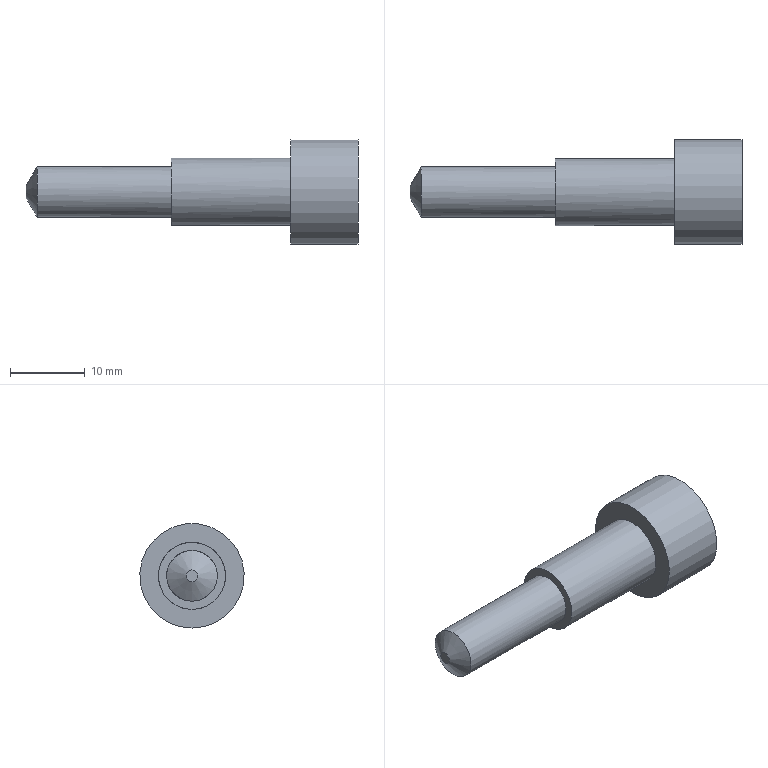Part | STEP file | solid 88 | 1 solid | 8 faces | box 44.5 x 14 x 14 mm | volume 3080 mm3 | plane 4 | cylinder 3 | cone 1 | commonest cylinder face diameters 6.8 x1 9 x1 14 x1